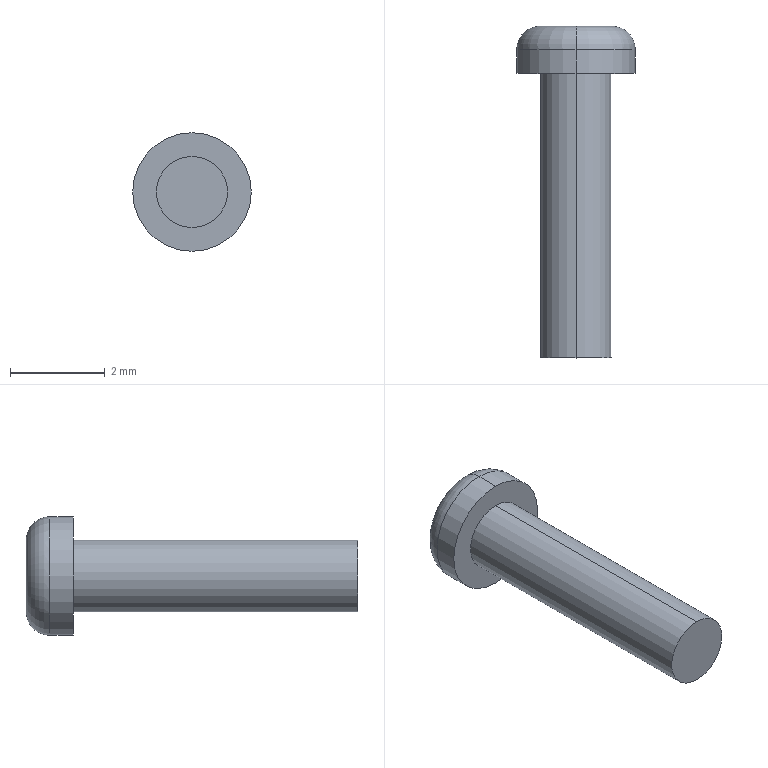Part | SolidWorks | features ICE 2, Extrusion 1, Fillet 1 | 1 solid | 16 faces | box 2.5 x 7 x 2.5 mm | volume 14.982 mm3 | plane 10 | cylinder 4 | torus 2 | commonest cylinder face diameters 1.5 x2 2.5 x2
STEP:
#1=CARTESIAN_POINT('',(0.,6.5,-1.25));
#2=VERTEX_POINT('',#1);
#3=CARTESIAN_POINT('',(0.,6.5,1.25));
#4=VERTEX_POINT('',#3);
#5=CARTESIAN_POINT('',(0.,6.5,0.));
#6=DIRECTION('',(0.,-1.,0.));
#7=DIRECTION('',(0.,0.,1.));
#8=AXIS2_PLACEMENT_3D('',#5,#6,#7);
#9=CIRCLE('',#8,1.25);
#10=EDGE_CURVE('',#2,#4,#9,.T.);
#11=ORIENTED_EDGE('',*,*,#10,.F.);
#12=CARTESIAN_POINT('',(0.,7.,-0.75));
#13=VERTEX_POINT('',#12);
#14=CARTESIAN_POINT('',(0.,6.5,-0.75));
#15=DIRECTION('',(1.,0.,0.));
#16=DIRECTION('',(0.,0.,-1.));
#17=AXIS2_PLACEMENT_3D('',#14,#15,#16);
#18=CIRCLE('',#17,0.5);
#19=EDGE_CURVE('',#2,#13,#18,.T.);
#20=ORIENTED_EDGE('',*,*,#19,.T.);
#21=CARTESIAN_POINT('',(0.,7.,0.75));
#22=VERTEX_POINT('',#21);
#23=CARTESIAN_POINT('',(0.,7.,0.));
#24=DIRECTION('',(0.,1.,0.));
#25=DIRECTION('',(0.,0.,1.));
#26=AXIS2_PLACEMENT_3D('',#23,#24,#25);
#27=CIRCLE('',#26,0.75);
#28=EDGE_CURVE('',#22,#13,#27,.T.);
#29=ORIENTED_EDGE('',*,*,#28,.F.);
#30=CARTESIAN_POINT('',(0.,6.5,0.75));
#31=DIRECTION('',(-1.,0.,0.));
#32=DIRECTION('',(0.,0.,1.));
#33=AXIS2_PLACEMENT_3D('',#30,#31,#32);
#34=CIRCLE('',#33,0.5);
#35=EDGE_CURVE('',#4,#22,#34,.T.);
#36=ORIENTED_EDGE('',*,*,#35,.F.);
#37=EDGE_LOOP('',(#11,#20,#29,#36));
#38=FACE_OUTER_BOUND('',#37,.T.);
#39=CARTESIAN_POINT('',(0.,6.5,0.));
#40=DIRECTION('',(0.,1.,0.));
#41=DIRECTION('',(0.,0.,1.));
#42=AXIS2_PLACEMENT_3D('',#39,#40,#41);
#43=TOROIDAL_SURFACE('',#42,0.75,0.5);
#44=ADVANCED_FACE('',(#38),#43,.T.);
#45=ORIENTED_EDGE('',*,*,#10,.T.);
#46=CARTESIAN_POINT('',(0.,6.,1.25));
#47=VERTEX_POINT('',#46);
#48=CARTESIAN_POINT('',(0.,7.,1.25));
#49=DIRECTION('',(0.,-1.,0.));
#50=VECTOR('',#49,1000.);
#51=LINE('',#48,#50);
#52=EDGE_CURVE('',#4,#47,#51,.T.);
#53=ORIENTED_EDGE('',*,*,#52,.T.);
#54=CARTESIAN_POINT('',(0.,6.,-1.25));
#55=VERTEX_POINT('',#54);
#56=CARTESIAN_POINT('',(0.,6.,0.));
#57=DIRECTION('',(0.,1.,0.));
#58=DIRECTION('',(0.,0.,1.));
#59=AXIS2_PLACEMENT_3D('',#56,#57,#58);
#60=CIRCLE('',#59,1.25);
#61=EDGE_CURVE('',#47,#55,#60,.T.);
#62=ORIENTED_EDGE('',*,*,#61,.T.);
#63=CARTESIAN_POINT('',(0.,7.,-1.25));
#64=DIRECTION('',(0.,-1.,0.));
#65=VECTOR('',#64,1000.);
#66=LINE('',#63,#65);
#67=EDGE_CURVE('',#2,#55,#66,.T.);
#68=ORIENTED_EDGE('',*,*,#67,.F.);
#69=EDGE_LOOP('',(#45,#53,#62,#68));
#70=FACE_OUTER_BOUND('',#69,.T.);
#71=CARTESIAN_POINT('',(0.,7.,0.));
#72=DIRECTION('',(0.,-1.,0.));
#73=DIRECTION('',(0.,0.,-1.));
#74=AXIS2_PLACEMENT_3D('',#71,#72,#73);
#75=CYLINDRICAL_SURFACE('',#74,1.25);
#76=ADVANCED_FACE('',(#70),#75,.T.);
#77=CARTESIAN_POINT('',(0.,6.,0.75));
#78=VERTEX_POINT('',#77);
#79=CARTESIAN_POINT('',(0.,6.,-0.75));
#80=VERTEX_POINT('',#79);
#81=CARTESIAN_POINT('',(0.,6.,0.));
#82=DIRECTION('',(0.,1.,0.));
#83=DIRECTION('',(0.,0.,1.));
#84=AXIS2_PLACEMENT_3D('',#81,#82,#83);
#85=CIRCLE('',#84,0.75);
#86=EDGE_CURVE('',#78,#80,#85,.T.);
#87=ORIENTED_EDGE('',*,*,#86,.F.);
#88=CARTESIAN_POINT('',(0.,0.,0.75));
#89=VERTEX_POINT('',#88);
#90=CARTESIAN_POINT('',(0.,6.,0.75));
#91=DIRECTION('',(0.,-1.,0.));
#92=VECTOR('',#91,1000.);
#93=LINE('',#90,#92);
#94=EDGE_CURVE('',#78,#89,#93,.T.);
#95=ORIENTED_EDGE('',*,*,#94,.T.);
#96=CARTESIAN_POINT('',(0.,0.,-0.75));
#97=VERTEX_POINT('',#96);
#98=CARTESIAN_POINT('',(0.,0.,0.));
#99=DIRECTION('',(0.,1.,0.));
#100=DIRECTION('',(0.,0.,1.));
#101=AXIS2_PLACEMENT_3D('',#98,#99,#100);
#102=CIRCLE('',#101,0.75);
#103=EDGE_CURVE('',#89,#97,#102,.T.);
#104=ORIENTED_EDGE('',*,*,#103,.T.);
#105=CARTESIAN_POINT('',(0.,6.,-0.75));
#106=DIRECTION('',(0.,-1.,0.));
#107=VECTOR('',#106,1000.);
#108=LINE('',#105,#107);
#109=EDGE_CURVE('',#80,#97,#108,.T.);
#110=ORIENTED_EDGE('',*,*,#109,.F.);
#111=EDGE_LOOP('',(#87,#95,#104,#110));
#112=FACE_OUTER_BOUND('',#111,.T.);
#113=CARTESIAN_POINT('',(0.,6.,0.));
#114=DIRECTION('',(0.,-1.,0.));
#115=DIRECTION('',(0.,0.,-1.));
#116=AXIS2_PLACEMENT_3D('',#113,#114,#115);
#117=CYLINDRICAL_SURFACE('',#116,0.75);
#118=ADVANCED_FACE('',(#112),#117,.T.);
#119=ORIENTED_EDGE('',*,*,#94,.F.);
#120=CARTESIAN_POINT('',(0.,6.,0.));
#121=DIRECTION('',(0.,1.,0.));
#122=DIRECTION('',(0.,0.,1.));
#123=AXIS2_PLACEMENT_3D('',#120,#121,#122);
#124=CIRCLE('',#123,0.75);
#125=EDGE_CURVE('',#80,#78,#124,.T.);
#126=ORIENTED_EDGE('',*,*,#125,.F.);
#127=ORIENTED_EDGE('',*,*,#109,.T.);
#128=CARTESIAN_POINT('',(0.,0.,0.));
#129=DIRECTION('',(0.,1.,0.));
#130=DIRECTION('',(0.,0.,1.));
#131=AXIS2_PLACEMENT_3D('',#128,#129,#130);
#132=CIRCLE('',#131,0.75);
#133=EDGE_CURVE('',#97,#89,#132,.T.);
#134=ORIENTED_EDGE('',*,*,#133,.T.);
#135=EDGE_LOOP('',(#119,#126,#127,#134));
#136=FACE_OUTER_BOUND('',#135,.T.);
#137=CARTESIAN_POINT('',(0.,6.,0.));
#138=DIRECTION('',(0.,-1.,0.));
#139=DIRECTION('',(0.,0.,-1.));
#140=AXIS2_PLACEMENT_3D('',#137,#138,#139);
#141=CYLINDRICAL_SURFACE('',#140,0.75);
#142=ADVANCED_FACE('',(#136),#141,.T.);
#143=ORIENTED_EDGE('',*,*,#133,.F.);
#144=ORIENTED_EDGE('',*,*,#103,.F.);
#145=EDGE_LOOP('',(#143,#144));
#146=FACE_OUTER_BOUND('',#145,.T.);
#147=CARTESIAN_POINT('',(0.,0.,0.));
#148=DIRECTION('',(0.,1.,0.));
#149=DIRECTION('',(0.,0.,1.));
#150=AXIS2_PLACEMENT_3D('',#147,#148,#149);
#151=PLANE('',#150);
#152=ADVANCED_FACE('',(#146),#151,.F.);
#153=ORIENTED_EDGE('',*,*,#52,.F.);
#154=CARTESIAN_POINT('',(0.,6.5,0.));
#155=DIRECTION('',(0.,-1.,0.));
#156=DIRECTION('',(0.,0.,1.));
#157=AXIS2_PLACEMENT_3D('',#154,#155,#156);
#158=CIRCLE('',#157,1.25);
#159=EDGE_CURVE('',#4,#2,#158,.T.);
#160=ORIENTED_EDGE('',*,*,#159,.T.);
#161=ORIENTED_EDGE('',*,*,#67,.T.);
#162=CARTESIAN_POINT('',(0.,6.,0.));
#163=DIRECTION('',(0.,1.,0.));
#164=DIRECTION('',(0.,0.,1.));
#165=AXIS2_PLACEMENT_3D('',#162,#163,#164);
#166=CIRCLE('',#165,1.25);
#167=EDGE_CURVE('',#55,#47,#166,.T.);
#168=ORIENTED_EDGE('',*,*,#167,.T.);
#169=EDGE_LOOP('',(#153,#160,#161,#168));
#170=FACE_OUTER_BOUND('',#169,.T.);
#171=CARTESIAN_POINT('',(0.,7.,0.));
#172=DIRECTION('',(0.,-1.,0.));
#173=DIRECTION('',(0.,0.,-1.));
#174=AXIS2_PLACEMENT_3D('',#171,#172,#173);
#175=CYLINDRICAL_SURFACE('',#174,1.25);
#176=ADVANCED_FACE('',(#170),#175,.T.);
#177=CARTESIAN_POINT('',(0.4589,7.,-0.2649));
#178=VERTEX_POINT('',#177);
#179=CARTESIAN_POINT('',(0.,7.,-0.5299));
#180=VERTEX_POINT('',#179);
#181=CARTESIAN_POINT('',(0.4589,7.,-0.2649));
#182=DIRECTION('',(-0.866,0.,-0.5));
#183=VECTOR('',#182,1000.);
#184=LINE('',#181,#183);
#185=EDGE_CURVE('',#178,#180,#184,.T.);
#186=ORIENTED_EDGE('',*,*,#185,.F.);
#187=CARTESIAN_POINT('',(0.4589,7.,0.2649));
#188=VERTEX_POINT('',#187);
#189=CARTESIAN_POINT('',(0.4589,7.,0.2649));
#190=DIRECTION('',(0.,0.,-1.));
#191=VECTOR('',#190,1000.);
#192=LINE('',#189,#191);
#193=EDGE_CURVE('',#188,#178,#192,.T.);
#194=ORIENTED_EDGE('',*,*,#193,.F.);
#195=CARTESIAN_POINT('',(0.,7.,0.5299));
#196=VERTEX_POINT('',#195);
#197=CARTESIAN_POINT('',(0.,7.,0.5299));
#198=DIRECTION('',(0.866,0.,-0.5));
#199=VECTOR('',#198,1000.);
#200=LINE('',#197,#199);
#201=EDGE_CURVE('',#196,#188,#200,.T.);
#202=ORIENTED_EDGE('',*,*,#201,.F.);
#203=CARTESIAN_POINT('',(-0.4589,7.,0.2649));
#204=VERTEX_POINT('',#203);
#205=CARTESIAN_POINT('',(-0.4589,7.,0.2649));
#206=DIRECTION('',(0.866,0.,0.5));
#207=VECTOR('',#206,1000.);
#208=LINE('',#205,#207);
#209=EDGE_CURVE('',#204,#196,#208,.T.);
#210=ORIENTED_EDGE('',*,*,#209,.F.);
#211=CARTESIAN_POINT('',(-0.4589,7.,-0.2649));
#212=VERTEX_POINT('',#211);
#213=CARTESIAN_POINT('',(-0.4589,7.,-0.2649));
#214=DIRECTION('',(0.,0.,1.));
#215=VECTOR('',#214,1000.);
#216=LINE('',#213,#215);
#217=EDGE_CURVE('',#212,#204,#216,.T.);
#218=ORIENTED_EDGE('',*,*,#217,.F.);
#219=CARTESIAN_POINT('',(0.,7.,-0.5299));
#220=DIRECTION('',(-0.866,0.,0.5));
#221=VECTOR('',#220,1000.);
#222=LINE('',#219,#221);
#223=EDGE_CURVE('',#180,#212,#222,.T.);
#224=ORIENTED_EDGE('',*,*,#223,.F.);
#225=EDGE_LOOP('',(#186,#194,#202,#210,#218,#224));
#226=FACE_BOUND('',#225,.T.);
#227=ORIENTED_EDGE('',*,*,#28,.T.);
#228=CARTESIAN_POINT('',(0.,7.,0.));
#229=DIRECTION('',(0.,1.,0.));
#230=DIRECTION('',(0.,0.,1.));
#231=AXIS2_PLACEMENT_3D('',#228,#229,#230);
#232=CIRCLE('',#231,0.75);
#233=EDGE_CURVE('',#13,#22,#232,.T.);
#234=ORIENTED_EDGE('',*,*,#233,.T.);
#235=EDGE_LOOP('',(#227,#234));
#236=FACE_OUTER_BOUND('',#235,.T.);
#237=CARTESIAN_POINT('',(0.,7.,0.));
#238=DIRECTION('',(0.,1.,0.));
#239=DIRECTION('',(0.,0.,1.));
#240=AXIS2_PLACEMENT_3D('',#237,#238,#239);
#241=PLANE('',#240);
#242=ADVANCED_FACE('',(#226,#236),#241,.T.);
#243=ORIENTED_EDGE('',*,*,#125,.T.);
#244=ORIENTED_EDGE('',*,*,#86,.T.);
#245=EDGE_LOOP('',(#243,#244));
#246=FACE_BOUND('',#245,.T.);
#247=ORIENTED_EDGE('',*,*,#167,.F.);
#248=ORIENTED_EDGE('',*,*,#61,.F.);
#249=EDGE_LOOP('',(#247,#248));
#250=FACE_OUTER_BOUND('',#249,.T.);
#251=CARTESIAN_POINT('',(0.,6.,0.));
#252=DIRECTION('',(0.,1.,0.));
#253=DIRECTION('',(0.,0.,1.));
#254=AXIS2_PLACEMENT_3D('',#251,#252,#253);
#255=PLANE('',#254);
#256=ADVANCED_FACE('',(#246,#250),#255,.F.);
#257=ORIENTED_EDGE('',*,*,#19,.F.);
#258=ORIENTED_EDGE('',*,*,#159,.F.);
#259=ORIENTED_EDGE('',*,*,#35,.T.);
#260=ORIENTED_EDGE('',*,*,#233,.F.);
#261=EDGE_LOOP('',(#257,#258,#259,#260));
#262=FACE_OUTER_BOUND('',#261,.T.);
#263=CARTESIAN_POINT('',(0.,6.5,0.));
#264=DIRECTION('',(0.,1.,0.));
#265=DIRECTION('',(0.,0.,1.));
#266=AXIS2_PLACEMENT_3D('',#263,#264,#265);
#267=TOROIDAL_SURFACE('',#266,0.75,0.5);
#268=ADVANCED_FACE('',(#262),#267,.T.);
#269=ORIENTED_EDGE('',*,*,#185,.T.);
#270=CARTESIAN_POINT('',(0.,6.8,-0.5299));
#271=VERTEX_POINT('',#270);
#272=CARTESIAN_POINT('',(0.,6.8,-0.5299));
#273=DIRECTION('',(0.,1.,0.));
#274=VECTOR('',#273,1000.);
#275=LINE('',#272,#274);
#276=EDGE_CURVE('',#271,#180,#275,.T.);
#277=ORIENTED_EDGE('',*,*,#276,.F.);
#278=CARTESIAN_POINT('',(0.4589,6.8,-0.2649));
#279=VERTEX_POINT('',#278);
#280=CARTESIAN_POINT('',(0.4589,6.8,-0.2649));
#281=DIRECTION('',(-0.866,0.,-0.5));
#282=VECTOR('',#281,1000.);
#283=LINE('',#280,#282);
#284=EDGE_CURVE('',#279,#271,#283,.T.);
#285=ORIENTED_EDGE('',*,*,#284,.F.);
#286=CARTESIAN_POINT('',(0.4589,6.8,-0.2649));
#287=DIRECTION('',(0.,1.,0.));
#288=VECTOR('',#287,1000.);
#289=LINE('',#286,#288);
#290=EDGE_CURVE('',#279,#178,#289,.T.);
#291=ORIENTED_EDGE('',*,*,#290,.T.);
#292=EDGE_LOOP('',(#269,#277,#285,#291));
#293=FACE_OUTER_BOUND('',#292,.T.);
#294=CARTESIAN_POINT('',(0.4589,6.8,-0.2649));
#295=DIRECTION('',(0.5,0.,-0.866));
#296=DIRECTION('',(-0.866,0.,-0.5));
#297=AXIS2_PLACEMENT_3D('',#294,#295,#296);
#298=PLANE('',#297);
#299=ADVANCED_FACE('',(#293),#298,.F.);
#300=ORIENTED_EDGE('',*,*,#193,.T.);
#301=ORIENTED_EDGE('',*,*,#290,.F.);
#302=CARTESIAN_POINT('',(0.4589,6.8,0.2649));
#303=VERTEX_POINT('',#302);
#304=CARTESIAN_POINT('',(0.4589,6.8,0.2649));
#305=DIRECTION('',(0.,0.,-1.));
#306=VECTOR('',#305,1000.);
#307=LINE('',#304,#306);
#308=EDGE_CURVE('',#303,#279,#307,.T.);
#309=ORIENTED_EDGE('',*,*,#308,.F.);
#310=CARTESIAN_POINT('',(0.4589,6.8,0.2649));
#311=DIRECTION('',(0.,1.,0.));
#312=VECTOR('',#311,1000.);
#313=LINE('',#310,#312);
#314=EDGE_CURVE('',#303,#188,#313,.T.);
#315=ORIENTED_EDGE('',*,*,#314,.T.);
#316=EDGE_LOOP('',(#300,#301,#309,#315));
#317=FACE_OUTER_BOUND('',#316,.T.);
#318=CARTESIAN_POINT('',(0.4589,6.8,0.2649));
#319=DIRECTION('',(1.,0.,0.));
#320=DIRECTION('',(0.,0.,-1.));
#321=AXIS2_PLACEMENT_3D('',#318,#319,#320);
#322=PLANE('',#321);
#323=ADVANCED_FACE('',(#317),#322,.F.);
#324=ORIENTED_EDGE('',*,*,#201,.T.);
#325=ORIENTED_EDGE('',*,*,#314,.F.);
#326=CARTESIAN_POINT('',(0.,6.8,0.5299));
#327=VERTEX_POINT('',#326);
#328=CARTESIAN_POINT('',(0.,6.8,0.5299));
#329=DIRECTION('',(0.866,0.,-0.5));
#330=VECTOR('',#329,1000.);
#331=LINE('',#328,#330);
#332=EDGE_CURVE('',#327,#303,#331,.T.);
#333=ORIENTED_EDGE('',*,*,#332,.F.);
#334=CARTESIAN_POINT('',(0.,6.8,0.5299));
#335=DIRECTION('',(0.,1.,0.));
#336=VECTOR('',#335,1000.);
#337=LINE('',#334,#336);
#338=EDGE_CURVE('',#327,#196,#337,.T.);
#339=ORIENTED_EDGE('',*,*,#338,.T.);
#340=EDGE_LOOP('',(#324,#325,#333,#339));
#341=FACE_OUTER_BOUND('',#340,.T.);
#342=CARTESIAN_POINT('',(0.,6.8,0.5299));
#343=DIRECTION('',(0.5,0.,0.866));
#344=DIRECTION('',(0.866,0.,-0.5));
#345=AXIS2_PLACEMENT_3D('',#342,#343,#344);
#346=PLANE('',#345);
#347=ADVANCED_FACE('',(#341),#346,.F.);
#348=ORIENTED_EDGE('',*,*,#209,.T.);
#349=ORIENTED_EDGE('',*,*,#338,.F.);
#350=CARTESIAN_POINT('',(-0.4589,6.8,0.2649));
#351=VERTEX_POINT('',#350);
#352=CARTESIAN_POINT('',(-0.4589,6.8,0.2649));
#353=DIRECTION('',(0.866,0.,0.5));
#354=VECTOR('',#353,1000.);
#355=LINE('',#352,#354);
#356=EDGE_CURVE('',#351,#327,#355,.T.);
#357=ORIENTED_EDGE('',*,*,#356,.F.);
#358=CARTESIAN_POINT('',(-0.4589,6.8,0.2649));
#359=DIRECTION('',(0.,1.,0.));
#360=VECTOR('',#359,1000.);
#361=LINE('',#358,#360);
#362=EDGE_CURVE('',#351,#204,#361,.T.);
#363=ORIENTED_EDGE('',*,*,#362,.T.);
#364=EDGE_LOOP('',(#348,#349,#357,#363));
#365=FACE_OUTER_BOUND('',#364,.T.);
#366=CARTESIAN_POINT('',(-0.4589,6.8,0.2649));
#367=DIRECTION('',(-0.5,0.,0.866));
#368=DIRECTION('',(0.866,0.,0.5));
#369=AXIS2_PLACEMENT_3D('',#366,#367,#368);
#370=PLANE('',#369);
#371=ADVANCED_FACE('',(#365),#370,.F.);
#372=ORIENTED_EDGE('',*,*,#217,.T.);
#373=ORIENTED_EDGE('',*,*,#362,.F.);
#374=CARTESIAN_POINT('',(-0.4589,6.8,-0.2649));
#375=VERTEX_POINT('',#374);
#376=CARTESIAN_POINT('',(-0.4589,6.8,-0.2649));
#377=DIRECTION('',(0.,0.,1.));
#378=VECTOR('',#377,1000.);
#379=LINE('',#376,#378);
#380=EDGE_CURVE('',#375,#351,#379,.T.);
#381=ORIENTED_EDGE('',*,*,#380,.F.);
#382=CARTESIAN_POINT('',(-0.4589,6.8,-0.2649));
#383=DIRECTION('',(0.,1.,0.));
#384=VECTOR('',#383,1000.);
#385=LINE('',#382,#384);
#386=EDGE_CURVE('',#375,#212,#385,.T.);
#387=ORIENTED_EDGE('',*,*,#386,.T.);
#388=EDGE_LOOP('',(#372,#373,#381,#387));
#389=FACE_OUTER_BOUND('',#388,.T.);
#390=CARTESIAN_POINT('',(-0.4589,6.8,-0.2649));
#391=DIRECTION('',(-1.,0.,0.));
#392=DIRECTION('',(0.,0.,1.));
#393=AXIS2_PLACEMENT_3D('',#390,#391,#392);
#394=PLANE('',#393);
#395=ADVANCED_FACE('',(#389),#394,.F.);
#396=ORIENTED_EDGE('',*,*,#223,.T.);
#397=ORIENTED_EDGE('',*,*,#386,.F.);
#398=CARTESIAN_POINT('',(0.,6.8,-0.5299));
#399=DIRECTION('',(-0.866,0.,0.5));
#400=VECTOR('',#399,1000.);
#401=LINE('',#398,#400);
#402=EDGE_CURVE('',#271,#375,#401,.T.);
#403=ORIENTED_EDGE('',*,*,#402,.F.);
#404=ORIENTED_EDGE('',*,*,#276,.T.);
#405=EDGE_LOOP('',(#396,#397,#403,#404));
#406=FACE_OUTER_BOUND('',#405,.T.);
#407=CARTESIAN_POINT('',(0.,6.8,-0.5299));
#408=DIRECTION('',(-0.5,0.,-0.866));
#409=DIRECTION('',(-0.866,0.,0.5));
#410=AXIS2_PLACEMENT_3D('',#407,#408,#409);
#411=PLANE('',#410);
#412=ADVANCED_FACE('',(#406),#411,.F.);
#413=ORIENTED_EDGE('',*,*,#284,.T.);
#414=ORIENTED_EDGE('',*,*,#402,.T.);
#415=ORIENTED_EDGE('',*,*,#380,.T.);
#416=ORIENTED_EDGE('',*,*,#356,.T.);
#417=ORIENTED_EDGE('',*,*,#332,.T.);
#418=ORIENTED_EDGE('',*,*,#308,.T.);
#419=EDGE_LOOP('',(#413,#414,#415,#416,#417,#418));
#420=FACE_OUTER_BOUND('',#419,.T.);
#421=CARTESIAN_POINT('',(0.,6.8,0.));
#422=DIRECTION('',(0.,1.,0.));
#423=DIRECTION('',(0.,0.,1.));
#424=AXIS2_PLACEMENT_3D('',#421,#422,#423);
#425=PLANE('',#424);
#426=ADVANCED_FACE('',(#420),#425,.T.);
#427=CLOSED_SHELL('',(#44,#76,#118,#142,#152,#176,#242,#256,#268,#299,#323,#347,#371,#395,#412,#426));
#428=MANIFOLD_SOLID_BREP('',#427);
#429=CARTESIAN_POINT('',(0.,0.,0.));
#430=DIRECTION('',(0.,0.,1.));
#431=DIRECTION('',(1.,0.,0.));
#432=AXIS2_PLACEMENT_3D('',#429,#430,#431);
#433=(LENGTH_UNIT()NAMED_UNIT(*)SI_UNIT(.MILLI.,.METRE.));
#434=UNCERTAINTY_MEASURE_WITH_UNIT(LENGTH_MEASURE(0.00001),#433,'','');
#435=(NAMED_UNIT(*)PLANE_ANGLE_UNIT()SI_UNIT($,.RADIAN.));
#436=(NAMED_UNIT(*)SI_UNIT($,.STERADIAN.)SOLID_ANGLE_UNIT());
#437=(GEOMETRIC_REPRESENTATION_CONTEXT(3)GLOBAL_UNCERTAINTY_ASSIGNED_CONTEXT((#434))GLOBAL_UNIT_ASSIGNED_CONTEXT((#433,#435,#436))REPRESENTATION_CONTEXT('',''));
#438=ADVANCED_BREP_SHAPE_REPRESENTATION('',(#428,#432),#437);